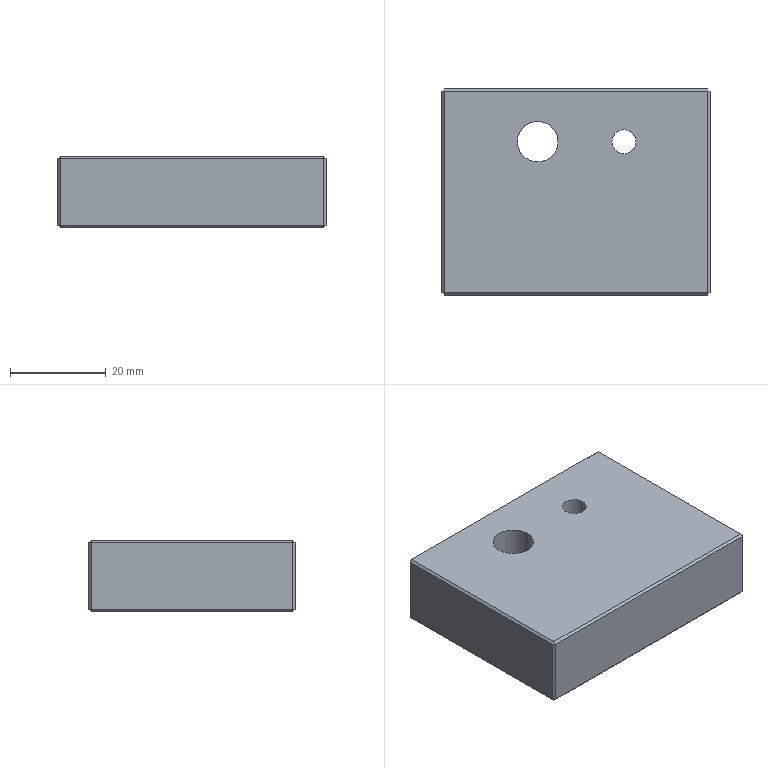Part | STEP file | 001-010-Waste limit block | 1 solid | 30 faces | box 56 x 43 x 15 mm | volume 34918 mm3 | plane 26 | cylinder 4 | commonest cylinder face diameters 5 x2 8.5 x2